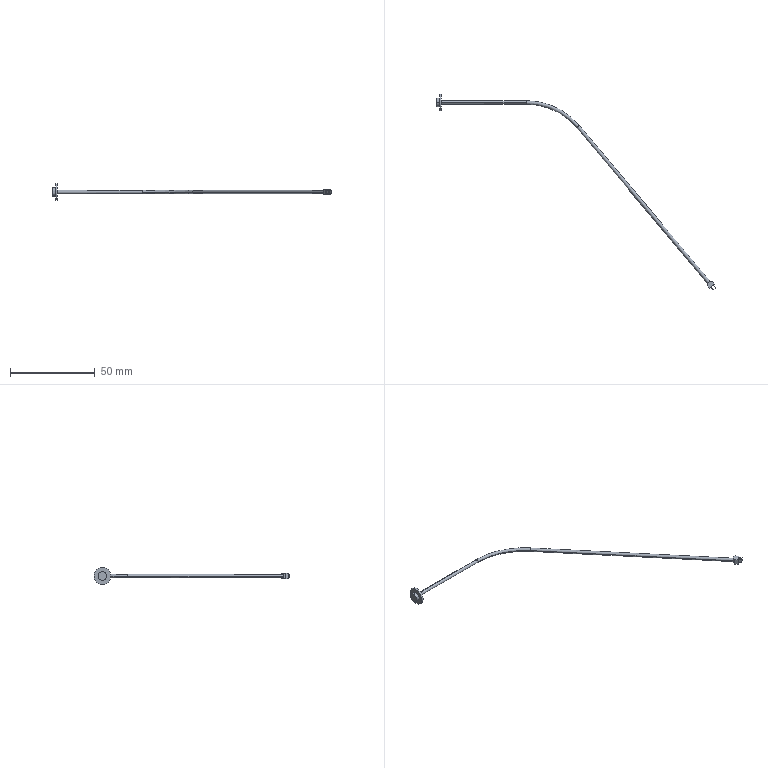Part | SolidWorks | features ICE 2, Revolution 1, Sweep 1 | 1 solid | 32 faces | box 164.795 x 115.719 x 10 mm | volume 796.943 mm3 | plane 22 | cylinder 8 | torus 2 | commonest cylinder face diameters 2 x4 5 x2 10 x2
STEP:
#1=CARTESIAN_POINT('',(53.,1.,0.));
#2=VERTEX_POINT('',#1);
#3=CARTESIAN_POINT('',(53.,0.,-1.));
#4=VERTEX_POINT('',#3);
#5=CARTESIAN_POINT('',(53.,0.,0.));
#6=DIRECTION('',(-1.,0.,0.));
#7=DIRECTION('',(0.,-1.,0.));
#8=AXIS2_PLACEMENT_3D('',#5,#6,#7);
#9=CIRCLE('',#8,1.);
#10=EDGE_CURVE('',#2,#4,#9,.T.);
#11=ORIENTED_EDGE('',*,*,#10,.F.);
#12=CARTESIAN_POINT('',(84.408,-13.646,0.));
#13=VERTEX_POINT('',#12);
#14=CARTESIAN_POINT('',(53.,-40.,0.));
#15=DIRECTION('',(0.,0.,-1.));
#16=DIRECTION('',(-1.,0.,0.));
#17=AXIS2_PLACEMENT_3D('',#14,#15,#16);
#18=CIRCLE('',#17,41.);
#19=EDGE_CURVE('',#2,#13,#18,.T.);
#20=ORIENTED_EDGE('',*,*,#19,.T.);
#21=CARTESIAN_POINT('',(82.876,-14.931,0.));
#22=VERTEX_POINT('',#21);
#23=CARTESIAN_POINT('',(83.642,-14.288,0.));
#24=DIRECTION('',(-0.6428,0.766,0.));
#25=DIRECTION('',(-0.766,-0.6428,0.));
#26=AXIS2_PLACEMENT_3D('',#23,#24,#25);
#27=CIRCLE('',#26,1.);
#28=EDGE_CURVE('',#13,#22,#27,.T.);
#29=ORIENTED_EDGE('',*,*,#28,.T.);
#30=CARTESIAN_POINT('',(53.,-1.,0.));
#31=VERTEX_POINT('',#30);
#32=CARTESIAN_POINT('',(53.,-40.,0.));
#33=DIRECTION('',(0.,0.,-1.));
#34=DIRECTION('',(-1.,0.,0.));
#35=AXIS2_PLACEMENT_3D('',#32,#33,#34);
#36=CIRCLE('',#35,39.);
#37=EDGE_CURVE('',#31,#22,#36,.T.);
#38=ORIENTED_EDGE('',*,*,#37,.F.);
#39=CARTESIAN_POINT('',(53.,0.,0.));
#40=DIRECTION('',(-1.,0.,0.));
#41=DIRECTION('',(0.,-1.,0.));
#42=AXIS2_PLACEMENT_3D('',#39,#40,#41);
#43=CIRCLE('',#42,1.);
#44=EDGE_CURVE('',#4,#31,#43,.T.);
#45=ORIENTED_EDGE('',*,*,#44,.F.);
#46=EDGE_LOOP('',(#11,#20,#29,#38,#45));
#47=FACE_OUTER_BOUND('',#46,.T.);
#48=CARTESIAN_POINT('',(53.,-40.,0.));
#49=DIRECTION('',(0.,0.,-1.));
#50=DIRECTION('',(-1.,0.,0.));
#51=AXIS2_PLACEMENT_3D('',#48,#49,#50);
#52=TOROIDAL_SURFACE('',#51,40.,1.);
#53=ADVANCED_FACE('',(#47),#52,.T.);
#54=CARTESIAN_POINT('',(83.642,-14.288,0.));
#55=DIRECTION('',(-0.6428,0.766,0.));
#56=DIRECTION('',(-0.766,-0.6428,0.));
#57=AXIS2_PLACEMENT_3D('',#54,#55,#56);
#58=CIRCLE('',#57,1.);
#59=EDGE_CURVE('',#22,#13,#58,.T.);
#60=ORIENTED_EDGE('',*,*,#59,.F.);
#61=CARTESIAN_POINT('',(160.01,-106.857,0.));
#62=VERTEX_POINT('',#61);
#63=CARTESIAN_POINT('',(82.876,-14.931,0.));
#64=DIRECTION('',(0.6428,-0.766,0.));
#65=VECTOR('',#64,1000.);
#66=LINE('',#63,#65);
#67=EDGE_CURVE('',#22,#62,#66,.T.);
#68=ORIENTED_EDGE('',*,*,#67,.T.);
#69=CARTESIAN_POINT('',(161.542,-105.571,0.));
#70=VERTEX_POINT('',#69);
#71=CARTESIAN_POINT('',(160.776,-106.214,0.));
#72=DIRECTION('',(-0.6428,0.766,0.));
#73=DIRECTION('',(-0.766,-0.6428,0.));
#74=AXIS2_PLACEMENT_3D('',#71,#72,#73);
#75=CIRCLE('',#74,1.);
#76=EDGE_CURVE('',#62,#70,#75,.T.);
#77=ORIENTED_EDGE('',*,*,#76,.T.);
#78=CARTESIAN_POINT('',(84.408,-13.646,0.));
#79=DIRECTION('',(0.6428,-0.766,0.));
#80=VECTOR('',#79,1000.);
#81=LINE('',#78,#80);
#82=EDGE_CURVE('',#13,#70,#81,.T.);
#83=ORIENTED_EDGE('',*,*,#82,.F.);
#84=EDGE_LOOP('',(#60,#68,#77,#83));
#85=FACE_OUTER_BOUND('',#84,.T.);
#86=CARTESIAN_POINT('',(83.642,-14.288,0.));
#87=DIRECTION('',(0.6428,-0.766,0.));
#88=DIRECTION('',(0.766,0.6428,0.));
#89=AXIS2_PLACEMENT_3D('',#86,#87,#88);
#90=CYLINDRICAL_SURFACE('',#89,1.);
#91=ADVANCED_FACE('',(#85),#90,.T.);
#92=CARTESIAN_POINT('',(3.,0.,1.));
#93=VERTEX_POINT('',#92);
#94=CARTESIAN_POINT('',(3.,0.,-1.));
#95=VERTEX_POINT('',#94);
#96=CARTESIAN_POINT('',(3.,0.,0.));
#97=DIRECTION('',(-1.,0.,0.));
#98=DIRECTION('',(0.,-1.,0.));
#99=AXIS2_PLACEMENT_3D('',#96,#97,#98);
#100=CIRCLE('',#99,1.);
#101=EDGE_CURVE('',#93,#95,#100,.T.);
#102=ORIENTED_EDGE('',*,*,#101,.F.);
#103=CARTESIAN_POINT('',(53.,0.,1.));
#104=VERTEX_POINT('',#103);
#105=CARTESIAN_POINT('',(3.,0.,1.));
#106=DIRECTION('',(1.,0.,0.));
#107=VECTOR('',#106,1000.);
#108=LINE('',#105,#107);
#109=EDGE_CURVE('',#93,#104,#108,.T.);
#110=ORIENTED_EDGE('',*,*,#109,.T.);
#111=CARTESIAN_POINT('',(53.,0.,0.));
#112=DIRECTION('',(-1.,0.,0.));
#113=DIRECTION('',(0.,-1.,0.));
#114=AXIS2_PLACEMENT_3D('',#111,#112,#113);
#115=CIRCLE('',#114,1.);
#116=EDGE_CURVE('',#104,#2,#115,.T.);
#117=ORIENTED_EDGE('',*,*,#116,.T.);
#118=ORIENTED_EDGE('',*,*,#10,.T.);
#119=CARTESIAN_POINT('',(3.,0.,-1.));
#120=DIRECTION('',(1.,0.,0.));
#121=VECTOR('',#120,1000.);
#122=LINE('',#119,#121);
#123=EDGE_CURVE('',#95,#4,#122,.T.);
#124=ORIENTED_EDGE('',*,*,#123,.F.);
#125=EDGE_LOOP('',(#102,#110,#117,#118,#124));
#126=FACE_OUTER_BOUND('',#125,.T.);
#127=CARTESIAN_POINT('',(3.,0.,0.));
#128=DIRECTION('',(1.,0.,0.));
#129=DIRECTION('',(0.,0.,-1.));
#130=AXIS2_PLACEMENT_3D('',#127,#128,#129);
#131=CYLINDRICAL_SURFACE('',#130,1.);
#132=ADVANCED_FACE('',(#126),#131,.T.);
#133=CARTESIAN_POINT('',(3.,0.,5.));
#134=VERTEX_POINT('',#133);
#135=CARTESIAN_POINT('',(3.,0.,-5.));
#136=VERTEX_POINT('',#135);
#137=CARTESIAN_POINT('',(3.,0.,0.));
#138=DIRECTION('',(-1.,0.,0.));
#139=DIRECTION('',(0.,0.,1.));
#140=AXIS2_PLACEMENT_3D('',#137,#138,#139);
#141=CIRCLE('',#140,5.);
#142=EDGE_CURVE('',#134,#136,#141,.T.);
#143=ORIENTED_EDGE('',*,*,#142,.T.);
#144=CARTESIAN_POINT('',(2.,0.,-5.));
#145=VERTEX_POINT('',#144);
#146=CARTESIAN_POINT('',(0.,0.,-5.));
#147=DIRECTION('',(-1.,0.,0.));
#148=VECTOR('',#147,1000.);
#149=LINE('',#146,#148);
#150=EDGE_CURVE('',#136,#145,#149,.T.);
#151=ORIENTED_EDGE('',*,*,#150,.T.);
#152=CARTESIAN_POINT('',(2.,0.,5.));
#153=VERTEX_POINT('',#152);
#154=CARTESIAN_POINT('',(2.,0.,0.));
#155=DIRECTION('',(-1.,0.,0.));
#156=DIRECTION('',(0.,0.,1.));
#157=AXIS2_PLACEMENT_3D('',#154,#155,#156);
#158=CIRCLE('',#157,5.);
#159=EDGE_CURVE('',#153,#145,#158,.T.);
#160=ORIENTED_EDGE('',*,*,#159,.F.);
#161=CARTESIAN_POINT('',(0.,0.,5.));
#162=DIRECTION('',(-1.,0.,0.));
#163=VECTOR('',#162,1000.);
#164=LINE('',#161,#163);
#165=EDGE_CURVE('',#134,#153,#164,.T.);
#166=ORIENTED_EDGE('',*,*,#165,.F.);
#167=EDGE_LOOP('',(#143,#151,#160,#166));
#168=FACE_OUTER_BOUND('',#167,.T.);
#169=CARTESIAN_POINT('',(0.,0.,0.));
#170=DIRECTION('',(-1.,0.,0.));
#171=DIRECTION('',(0.,0.,1.));
#172=AXIS2_PLACEMENT_3D('',#169,#170,#171);
#173=CYLINDRICAL_SURFACE('',#172,5.);
#174=ADVANCED_FACE('',(#168),#173,.T.);
#175=CARTESIAN_POINT('',(2.,0.,2.5));
#176=VERTEX_POINT('',#175);
#177=CARTESIAN_POINT('',(2.,0.,-2.5));
#178=VERTEX_POINT('',#177);
#179=CARTESIAN_POINT('',(2.,0.,0.));
#180=DIRECTION('',(-1.,0.,0.));
#181=DIRECTION('',(0.,0.,1.));
#182=AXIS2_PLACEMENT_3D('',#179,#180,#181);
#183=CIRCLE('',#182,2.5);
#184=EDGE_CURVE('',#176,#178,#183,.T.);
#185=ORIENTED_EDGE('',*,*,#184,.T.);
#186=CARTESIAN_POINT('',(0.,0.,-2.5));
#187=VERTEX_POINT('',#186);
#188=CARTESIAN_POINT('',(0.,0.,-2.5));
#189=DIRECTION('',(-1.,0.,0.));
#190=VECTOR('',#189,1000.);
#191=LINE('',#188,#190);
#192=EDGE_CURVE('',#178,#187,#191,.T.);
#193=ORIENTED_EDGE('',*,*,#192,.T.);
#194=CARTESIAN_POINT('',(0.,0.,2.5));
#195=VERTEX_POINT('',#194);
#196=CARTESIAN_POINT('',(0.,0.,0.));
#197=DIRECTION('',(-1.,0.,0.));
#198=DIRECTION('',(0.,0.,1.));
#199=AXIS2_PLACEMENT_3D('',#196,#197,#198);
#200=CIRCLE('',#199,2.5);
#201=EDGE_CURVE('',#195,#187,#200,.T.);
#202=ORIENTED_EDGE('',*,*,#201,.F.);
#203=CARTESIAN_POINT('',(0.,0.,2.5));
#204=DIRECTION('',(-1.,0.,0.));
#205=VECTOR('',#204,1000.);
#206=LINE('',#203,#205);
#207=EDGE_CURVE('',#176,#195,#206,.T.);
#208=ORIENTED_EDGE('',*,*,#207,.F.);
#209=EDGE_LOOP('',(#185,#193,#202,#208));
#210=FACE_OUTER_BOUND('',#209,.T.);
#211=CARTESIAN_POINT('',(0.,0.,0.));
#212=DIRECTION('',(-1.,0.,0.));
#213=DIRECTION('',(0.,0.,1.));
#214=AXIS2_PLACEMENT_3D('',#211,#212,#213);
#215=CYLINDRICAL_SURFACE('',#214,2.5);
#216=ADVANCED_FACE('',(#210),#215,.T.);
#217=CARTESIAN_POINT('',(161.9,-109.187,1.));
#218=VERTEX_POINT('',#217);
#219=CARTESIAN_POINT('',(161.9,-109.187,-1.));
#220=VERTEX_POINT('',#219);
#221=CARTESIAN_POINT('',(161.9,-109.187,1.));
#222=DIRECTION('',(0.,0.,-1.));
#223=VECTOR('',#222,1000.);
#224=LINE('',#221,#223);
#225=EDGE_CURVE('',#218,#220,#224,.T.);
#226=ORIENTED_EDGE('',*,*,#225,.F.);
#227=CARTESIAN_POINT('',(162.13,-108.994,1.));
#228=VERTEX_POINT('',#227);
#229=CARTESIAN_POINT('',(162.13,-108.994,1.));
#230=DIRECTION('',(-0.766,-0.6428,0.));
#231=VECTOR('',#230,1000.);
#232=LINE('',#229,#231);
#233=EDGE_CURVE('',#228,#218,#232,.T.);
#234=ORIENTED_EDGE('',*,*,#233,.F.);
#235=CARTESIAN_POINT('',(162.13,-108.994,-1.));
#236=VERTEX_POINT('',#235);
#237=CARTESIAN_POINT('',(162.13,-108.994,1.));
#238=DIRECTION('',(0.,0.,-1.));
#239=VECTOR('',#238,1000.);
#240=LINE('',#237,#239);
#241=EDGE_CURVE('',#228,#236,#240,.T.);
#242=ORIENTED_EDGE('',*,*,#241,.T.);
#243=CARTESIAN_POINT('',(162.13,-108.994,-1.));
#244=DIRECTION('',(-0.766,-0.6428,0.));
#245=VECTOR('',#244,1000.);
#246=LINE('',#243,#245);
#247=EDGE_CURVE('',#236,#220,#246,.T.);
#248=ORIENTED_EDGE('',*,*,#247,.T.);
#249=EDGE_LOOP('',(#226,#234,#242,#248));
#250=FACE_BOUND('',#249,.T.);
#251=CARTESIAN_POINT('',(161.173,-109.798,-1.5));
#252=VERTEX_POINT('',#251);
#253=CARTESIAN_POINT('',(164.237,-107.226,-1.5));
#254=VERTEX_POINT('',#253);
#255=CARTESIAN_POINT('',(164.237,-107.226,-1.5));
#256=DIRECTION('',(0.766,0.6428,0.));
#257=VECTOR('',#256,1000.);
#258=LINE('',#255,#257);
#259=EDGE_CURVE('',#252,#254,#258,.T.);
#260=ORIENTED_EDGE('',*,*,#259,.T.);
#261=CARTESIAN_POINT('',(164.237,-107.226,1.5));
#262=VERTEX_POINT('',#261);
#263=CARTESIAN_POINT('',(164.237,-107.226,1.5));
#264=DIRECTION('',(0.,0.,-1.));
#265=VECTOR('',#264,1000.);
#266=LINE('',#263,#265);
#267=EDGE_CURVE('',#262,#254,#266,.T.);
#268=ORIENTED_EDGE('',*,*,#267,.F.);
#269=CARTESIAN_POINT('',(161.173,-109.798,1.5));
#270=VERTEX_POINT('',#269);
#271=CARTESIAN_POINT('',(164.237,-107.226,1.5));
#272=DIRECTION('',(0.766,0.6428,0.));
#273=VECTOR('',#272,1000.);
#274=LINE('',#271,#273);
#275=EDGE_CURVE('',#270,#262,#274,.T.);
#276=ORIENTED_EDGE('',*,*,#275,.F.);
#277=CARTESIAN_POINT('',(161.173,-109.798,1.5));
#278=DIRECTION('',(0.,0.,-1.));
#279=VECTOR('',#278,1000.);
#280=LINE('',#277,#279);
#281=EDGE_CURVE('',#270,#252,#280,.T.);
#282=ORIENTED_EDGE('',*,*,#281,.T.);
#283=EDGE_LOOP('',(#260,#268,#276,#282));
#284=FACE_OUTER_BOUND('',#283,.T.);
#285=CARTESIAN_POINT('',(163.509,-107.837,1.));
#286=VERTEX_POINT('',#285);
#287=CARTESIAN_POINT('',(163.279,-108.03,1.));
#288=VERTEX_POINT('',#287);
#289=CARTESIAN_POINT('',(163.279,-108.03,1.));
#290=DIRECTION('',(-0.766,-0.6428,0.));
#291=VECTOR('',#290,1000.);
#292=LINE('',#289,#291);
#293=EDGE_CURVE('',#286,#288,#292,.T.);
#294=ORIENTED_EDGE('',*,*,#293,.F.);
#295=CARTESIAN_POINT('',(163.509,-107.837,-1.));
#296=VERTEX_POINT('',#295);
#297=CARTESIAN_POINT('',(163.509,-107.837,1.));
#298=DIRECTION('',(0.,0.,-1.));
#299=VECTOR('',#298,1000.);
#300=LINE('',#297,#299);
#301=EDGE_CURVE('',#286,#296,#300,.T.);
#302=ORIENTED_EDGE('',*,*,#301,.T.);
#303=CARTESIAN_POINT('',(163.279,-108.03,-1.));
#304=VERTEX_POINT('',#303);
#305=CARTESIAN_POINT('',(163.279,-108.03,-1.));
#306=DIRECTION('',(-0.766,-0.6428,0.));
#307=VECTOR('',#306,1000.);
#308=LINE('',#305,#307);
#309=EDGE_CURVE('',#296,#304,#308,.T.);
#310=ORIENTED_EDGE('',*,*,#309,.T.);
#311=CARTESIAN_POINT('',(163.279,-108.03,1.));
#312=DIRECTION('',(0.,0.,-1.));
#313=VECTOR('',#312,1000.);
#314=LINE('',#311,#313);
#315=EDGE_CURVE('',#288,#304,#314,.T.);
#316=ORIENTED_EDGE('',*,*,#315,.F.);
#317=EDGE_LOOP('',(#294,#302,#310,#316));
#318=FACE_BOUND('',#317,.T.);
#319=CARTESIAN_POINT('',(164.237,-107.226,1.5));
#320=DIRECTION('',(-0.6428,0.766,0.));
#321=DIRECTION('',(-0.766,-0.6428,0.));
#322=AXIS2_PLACEMENT_3D('',#319,#320,#321);
#323=PLANE('',#322);
#324=ADVANCED_FACE('',(#250,#284,#318),#323,.F.);
#325=ORIENTED_EDGE('',*,*,#201,.T.);
#326=CARTESIAN_POINT('',(0.,0.,0.));
#327=DIRECTION('',(-1.,0.,0.));
#328=DIRECTION('',(0.,0.,1.));
#329=AXIS2_PLACEMENT_3D('',#326,#327,#328);
#330=CIRCLE('',#329,2.5);
#331=EDGE_CURVE('',#187,#195,#330,.T.);
#332=ORIENTED_EDGE('',*,*,#331,.T.);
#333=EDGE_LOOP('',(#325,#332));
#334=FACE_OUTER_BOUND('',#333,.T.);
#335=CARTESIAN_POINT('',(0.,0.,0.));
#336=DIRECTION('',(1.,0.,0.));
#337=DIRECTION('',(0.,0.,-1.));
#338=AXIS2_PLACEMENT_3D('',#335,#336,#337);
#339=PLANE('',#338);
#340=ADVANCED_FACE('',(#334),#339,.F.);
#341=ORIENTED_EDGE('',*,*,#192,.F.);
#342=CARTESIAN_POINT('',(2.,0.,0.));
#343=DIRECTION('',(-1.,0.,0.));
#344=DIRECTION('',(0.,0.,1.));
#345=AXIS2_PLACEMENT_3D('',#342,#343,#344);
#346=CIRCLE('',#345,2.5);
#347=EDGE_CURVE('',#178,#176,#346,.T.);
#348=ORIENTED_EDGE('',*,*,#347,.T.);
#349=ORIENTED_EDGE('',*,*,#207,.T.);
#350=ORIENTED_EDGE('',*,*,#331,.F.);
#351=EDGE_LOOP('',(#341,#348,#349,#350));
#352=FACE_OUTER_BOUND('',#351,.T.);
#353=CARTESIAN_POINT('',(0.,0.,0.));
#354=DIRECTION('',(-1.,0.,0.));
#355=DIRECTION('',(0.,0.,1.));
#356=AXIS2_PLACEMENT_3D('',#353,#354,#355);
#357=CYLINDRICAL_SURFACE('',#356,2.5);
#358=ADVANCED_FACE('',(#352),#357,.T.);
#359=ORIENTED_EDGE('',*,*,#184,.F.);
#360=ORIENTED_EDGE('',*,*,#347,.F.);
#361=EDGE_LOOP('',(#359,#360));
#362=FACE_BOUND('',#361,.T.);
#363=ORIENTED_EDGE('',*,*,#159,.T.);
#364=CARTESIAN_POINT('',(2.,0.,0.));
#365=DIRECTION('',(-1.,0.,0.));
#366=DIRECTION('',(0.,0.,1.));
#367=AXIS2_PLACEMENT_3D('',#364,#365,#366);
#368=CIRCLE('',#367,5.);
#369=EDGE_CURVE('',#145,#153,#368,.T.);
#370=ORIENTED_EDGE('',*,*,#369,.T.);
#371=EDGE_LOOP('',(#363,#370));
#372=FACE_OUTER_BOUND('',#371,.T.);
#373=CARTESIAN_POINT('',(2.,2.5,0.));
#374=DIRECTION('',(1.,0.,0.));
#375=DIRECTION('',(0.,0.,-1.));
#376=AXIS2_PLACEMENT_3D('',#373,#374,#375);
#377=PLANE('',#376);
#378=ADVANCED_FACE('',(#362,#372),#377,.F.);
#379=ORIENTED_EDGE('',*,*,#150,.F.);
#380=CARTESIAN_POINT('',(3.,0.,0.));
#381=DIRECTION('',(-1.,0.,0.));
#382=DIRECTION('',(0.,0.,1.));
#383=AXIS2_PLACEMENT_3D('',#380,#381,#382);
#384=CIRCLE('',#383,5.);
#385=EDGE_CURVE('',#136,#134,#384,.T.);
#386=ORIENTED_EDGE('',*,*,#385,.T.);
#387=ORIENTED_EDGE('',*,*,#165,.T.);
#388=ORIENTED_EDGE('',*,*,#369,.F.);
#389=EDGE_LOOP('',(#379,#386,#387,#388));
#390=FACE_OUTER_BOUND('',#389,.T.);
#391=CARTESIAN_POINT('',(0.,0.,0.));
#392=DIRECTION('',(-1.,0.,0.));
#393=DIRECTION('',(0.,0.,1.));
#394=AXIS2_PLACEMENT_3D('',#391,#392,#393);
#395=CYLINDRICAL_SURFACE('',#394,5.);
#396=ADVANCED_FACE('',(#390),#395,.T.);
#397=CARTESIAN_POINT('',(3.,0.,0.));
#398=DIRECTION('',(-1.,0.,0.));
#399=DIRECTION('',(0.,-1.,0.));
#400=AXIS2_PLACEMENT_3D('',#397,#398,#399);
#401=CIRCLE('',#400,1.);
#402=EDGE_CURVE('',#95,#93,#401,.T.);
#403=ORIENTED_EDGE('',*,*,#402,.T.);
#404=ORIENTED_EDGE('',*,*,#101,.T.);
#405=EDGE_LOOP('',(#403,#404));
#406=FACE_BOUND('',#405,.T.);
#407=ORIENTED_EDGE('',*,*,#142,.F.);
#408=ORIENTED_EDGE('',*,*,#385,.F.);
#409=EDGE_LOOP('',(#407,#408));
#410=FACE_OUTER_BOUND('',#409,.T.);
#411=CARTESIAN_POINT('',(3.,5.,0.));
#412=DIRECTION('',(-1.,0.,0.));
#413=DIRECTION('',(0.,0.,1.));
#414=AXIS2_PLACEMENT_3D('',#411,#412,#413);
#415=PLANE('',#414);
#416=ADVANCED_FACE('',(#406,#410),#415,.F.);
#417=ORIENTED_EDGE('',*,*,#67,.F.);
#418=ORIENTED_EDGE('',*,*,#28,.F.);
#419=ORIENTED_EDGE('',*,*,#82,.T.);
#420=CARTESIAN_POINT('',(160.776,-106.214,0.));
#421=DIRECTION('',(-0.6428,0.766,0.));
#422=DIRECTION('',(-0.766,-0.6428,0.));
#423=AXIS2_PLACEMENT_3D('',#420,#421,#422);
#424=CIRCLE('',#423,1.);
#425=EDGE_CURVE('',#70,#62,#424,.T.);
#426=ORIENTED_EDGE('',*,*,#425,.T.);
#427=EDGE_LOOP('',(#417,#418,#419,#426));
#428=FACE_OUTER_BOUND('',#427,.T.);
#429=CARTESIAN_POINT('',(83.642,-14.288,0.));
#430=DIRECTION('',(0.6428,-0.766,0.));
#431=DIRECTION('',(0.766,0.6428,0.));
#432=AXIS2_PLACEMENT_3D('',#429,#430,#431);
#433=CYLINDRICAL_SURFACE('',#432,1.);
#434=ADVANCED_FACE('',(#428),#433,.T.);
#435=ORIENTED_EDGE('',*,*,#19,.F.);
#436=ORIENTED_EDGE('',*,*,#116,.F.);
#437=CARTESIAN_POINT('',(53.,0.,0.));
#438=DIRECTION('',(-1.,0.,0.));
#439=DIRECTION('',(0.,-1.,0.));
#440=AXIS2_PLACEMENT_3D('',#437,#438,#439);
#441=CIRCLE('',#440,1.);
#442=EDGE_CURVE('',#31,#104,#441,.T.);
#443=ORIENTED_EDGE('',*,*,#442,.F.);
#444=ORIENTED_EDGE('',*,*,#37,.T.);
#445=ORIENTED_EDGE('',*,*,#59,.T.);
#446=EDGE_LOOP('',(#435,#436,#443,#444,#445));
#447=FACE_OUTER_BOUND('',#446,.T.);
#448=CARTESIAN_POINT('',(53.,-40.,0.));
#449=DIRECTION('',(0.,0.,-1.));
#450=DIRECTION('',(-1.,0.,0.));
#451=AXIS2_PLACEMENT_3D('',#448,#449,#450);
#452=TOROIDAL_SURFACE('',#451,40.,1.);
#453=ADVANCED_FACE('',(#447),#452,.T.);
#454=ORIENTED_EDGE('',*,*,#109,.F.);
#455=ORIENTED_EDGE('',*,*,#402,.F.);
#456=ORIENTED_EDGE('',*,*,#123,.T.);
#457=ORIENTED_EDGE('',*,*,#44,.T.);
#458=ORIENTED_EDGE('',*,*,#442,.T.);
#459=EDGE_LOOP('',(#454,#455,#456,#457,#458));
#460=FACE_OUTER_BOUND('',#459,.T.);
#461=CARTESIAN_POINT('',(3.,0.,0.));
#462=DIRECTION('',(1.,0.,0.));
#463=DIRECTION('',(0.,0.,-1.));
#464=AXIS2_PLACEMENT_3D('',#461,#462,#463);
#465=CYLINDRICAL_SURFACE('',#464,1.);
#466=ADVANCED_FACE('',(#460),#465,.T.);
#467=ORIENTED_EDGE('',*,*,#76,.F.);
#468=CARTESIAN_POINT('',(160.01,-106.857,1.5));
#469=VERTEX_POINT('',#468);
#470=CARTESIAN_POINT('',(160.01,-106.857,1.5));
#471=DIRECTION('',(0.,0.,-1.));
#472=VECTOR('',#471,1000.);
#473=LINE('',#470,#472);
#474=EDGE_CURVE('',#469,#62,#473,.T.);
#475=ORIENTED_EDGE('',*,*,#474,.F.);
#476=CARTESIAN_POINT('',(161.542,-105.571,1.5));
#477=VERTEX_POINT('',#476);
#478=CARTESIAN_POINT('',(160.01,-106.857,1.5));
#479=DIRECTION('',(-0.766,-0.6428,0.));
#480=VECTOR('',#479,1000.);
#481=LINE('',#478,#480);
#482=EDGE_CURVE('',#477,#469,#481,.T.);
#483=ORIENTED_EDGE('',*,*,#482,.F.);
#484=CARTESIAN_POINT('',(161.542,-105.571,1.5));
#485=DIRECTION('',(0.,0.,-1.));
#486=VECTOR('',#485,1000.);
#487=LINE('',#484,#486);
#488=EDGE_CURVE('',#477,#70,#487,.T.);
#489=ORIENTED_EDGE('',*,*,#488,.T.);
#490=EDGE_LOOP('',(#467,#475,#483,#489));
#491=FACE_OUTER_BOUND('',#490,.T.);
#492=CARTESIAN_POINT('',(160.01,-106.857,1.5));
#493=DIRECTION('',(0.6428,-0.766,0.));
#494=DIRECTION('',(0.766,0.6428,0.));
#495=AXIS2_PLACEMENT_3D('',#492,#493,#494);
#496=PLANE('',#495);
#497=ADVANCED_FACE('',(#491),#496,.F.);
#498=CARTESIAN_POINT('',(162.951,-105.694,-1.5));
#499=VERTEX_POINT('',#498);
#500=CARTESIAN_POINT('',(161.542,-105.571,-1.5));
#501=VERTEX_POINT('',#500);
#502=CARTESIAN_POINT('',(161.542,-105.571,-1.5));
#503=DIRECTION('',(-0.9962,0.08716,0.));
#504=VECTOR('',#503,1000.);
#505=LINE('',#502,#504);
#506=EDGE_CURVE('',#499,#501,#505,.T.);
#507=ORIENTED_EDGE('',*,*,#506,.T.);
#508=CARTESIAN_POINT('',(161.542,-105.571,1.5));
#509=DIRECTION('',(0.,0.,-1.));
#510=VECTOR('',#509,1000.);
#511=LINE('',#508,#510);
#512=EDGE_CURVE('',#70,#501,#511,.T.);
#513=ORIENTED_EDGE('',*,*,#512,.F.);
#514=ORIENTED_EDGE('',*,*,#488,.F.);
#515=CARTESIAN_POINT('',(162.951,-105.694,1.5));
#516=VERTEX_POINT('',#515);
#517=CARTESIAN_POINT('',(161.542,-105.571,1.5));
#518=DIRECTION('',(-0.9962,0.08716,0.));
#519=VECTOR('',#518,1000.);
#520=LINE('',#517,#519);
#521=EDGE_CURVE('',#516,#477,#520,.T.);
#522=ORIENTED_EDGE('',*,*,#521,.F.);
#523=CARTESIAN_POINT('',(162.951,-105.694,1.5));
#524=DIRECTION('',(0.,0.,-1.));
#525=VECTOR('',#524,1000.);
#526=LINE('',#523,#525);
#527=EDGE_CURVE('',#516,#499,#526,.T.);
#528=ORIENTED_EDGE('',*,*,#527,.T.);
#529=EDGE_LOOP('',(#507,#513,#514,#522,#528));
#530=FACE_OUTER_BOUND('',#529,.T.);
#531=CARTESIAN_POINT('',(161.542,-105.571,1.5));
#532=DIRECTION('',(-0.08716,-0.9962,0.));
#533=DIRECTION('',(0.9962,-0.08716,0.));
#534=AXIS2_PLACEMENT_3D('',#531,#532,#533);
#535=PLANE('',#534);
#536=ADVANCED_FACE('',(#530),#535,.F.);
#537=ORIENTED_EDGE('',*,*,#425,.F.);
#538=ORIENTED_EDGE('',*,*,#512,.T.);
#539=CARTESIAN_POINT('',(160.01,-106.857,-1.5));
#540=VERTEX_POINT('',#539);
#541=CARTESIAN_POINT('',(160.01,-106.857,-1.5));
#542=DIRECTION('',(-0.766,-0.6428,0.));
#543=VECTOR('',#542,1000.);
#544=LINE('',#541,#543);
#545=EDGE_CURVE('',#501,#540,#544,.T.);
#546=ORIENTED_EDGE('',*,*,#545,.T.);
#547=CARTESIAN_POINT('',(160.01,-106.857,1.5));
#548=DIRECTION('',(0.,0.,-1.));
#549=VECTOR('',#548,1000.);
#550=LINE('',#547,#549);
#551=EDGE_CURVE('',#62,#540,#550,.T.);
#552=ORIENTED_EDGE('',*,*,#551,.F.);
#553=EDGE_LOOP('',(#537,#538,#546,#552));
#554=FACE_OUTER_BOUND('',#553,.T.);
#555=CARTESIAN_POINT('',(160.01,-106.857,1.5));
#556=DIRECTION('',(0.6428,-0.766,0.));
#557=DIRECTION('',(0.766,0.6428,0.));
#558=AXIS2_PLACEMENT_3D('',#555,#556,#557);
#559=PLANE('',#558);
#560=ADVANCED_FACE('',(#554),#559,.F.);
#561=CARTESIAN_POINT('',(159.887,-108.265,-1.5));
#562=VERTEX_POINT('',#561);
#563=CARTESIAN_POINT('',(160.01,-106.857,-1.5));
#564=DIRECTION('',(-0.08716,-0.9962,0.));
#565=VECTOR('',#564,1000.);
#566=LINE('',#563,#565);
#567=EDGE_CURVE('',#540,#562,#566,.T.);
#568=ORIENTED_EDGE('',*,*,#567,.T.);
#569=CARTESIAN_POINT('',(159.887,-108.265,1.5));
#570=VERTEX_POINT('',#569);
#571=CARTESIAN_POINT('',(159.887,-108.265,1.5));
#572=DIRECTION('',(0.,0.,-1.));
#573=VECTOR('',#572,1000.);
#574=LINE('',#571,#573);
#575=EDGE_CURVE('',#570,#562,#574,.T.);
#576=ORIENTED_EDGE('',*,*,#575,.F.);
#577=CARTESIAN_POINT('',(160.01,-106.857,1.5));
#578=DIRECTION('',(-0.08716,-0.9962,0.));
#579=VECTOR('',#578,1000.);
#580=LINE('',#577,#579);
#581=EDGE_CURVE('',#469,#570,#580,.T.);
#582=ORIENTED_EDGE('',*,*,#581,.F.);
#583=ORIENTED_EDGE('',*,*,#474,.T.);
#584=ORIENTED_EDGE('',*,*,#551,.T.);
#585=EDGE_LOOP('',(#568,#576,#582,#583,#584));
#586=FACE_OUTER_BOUND('',#585,.T.);
#587=CARTESIAN_POINT('',(160.01,-106.857,1.5));
#588=DIRECTION('',(0.9962,-0.08716,0.));
#589=DIRECTION('',(0.08716,0.9962,0.));
#590=AXIS2_PLACEMENT_3D('',#587,#588,#589);
#591=PLANE('',#590);
#592=ADVANCED_FACE('',(#586),#591,.F.);
#593=CARTESIAN_POINT('',(159.887,-108.265,-1.5));
#594=DIRECTION('',(0.6428,-0.766,0.));
#595=VECTOR('',#594,1000.);
#596=LINE('',#593,#595);
#597=EDGE_CURVE('',#562,#252,#596,.T.);
#598=ORIENTED_EDGE('',*,*,#597,.T.);
#599=ORIENTED_EDGE('',*,*,#281,.F.);
#600=CARTESIAN_POINT('',(159.887,-108.265,1.5));
#601=DIRECTION('',(0.6428,-0.766,0.));
#602=VECTOR('',#601,1000.);
#603=LINE('',#600,#602);
#604=EDGE_CURVE('',#570,#270,#603,.T.);
#605=ORIENTED_EDGE('',*,*,#604,.F.);
#606=ORIENTED_EDGE('',*,*,#575,.T.);
#607=EDGE_LOOP('',(#598,#599,#605,#606));
#608=FACE_OUTER_BOUND('',#607,.T.);
#609=CARTESIAN_POINT('',(159.887,-108.265,1.5));
#610=DIRECTION('',(0.766,0.6428,0.));
#611=DIRECTION('',(-0.6428,0.766,0.));
#612=AXIS2_PLACEMENT_3D('',#609,#610,#611);
#613=PLANE('',#612);
#614=ADVANCED_FACE('',(#608),#613,.F.);
#615=CARTESIAN_POINT('',(162.951,-105.694,-1.5));
#616=DIRECTION('',(-0.6428,0.766,0.));
#617=VECTOR('',#616,1000.);
#618=LINE('',#615,#617);
#619=EDGE_CURVE('',#254,#499,#618,.T.);
#620=ORIENTED_EDGE('',*,*,#619,.T.);
#621=ORIENTED_EDGE('',*,*,#527,.F.);
#622=CARTESIAN_POINT('',(162.951,-105.694,1.5));
#623=DIRECTION('',(-0.6428,0.766,0.));
#624=VECTOR('',#623,1000.);
#625=LINE('',#622,#624);
#626=EDGE_CURVE('',#262,#516,#625,.T.);
#627=ORIENTED_EDGE('',*,*,#626,.F.);
#628=ORIENTED_EDGE('',*,*,#267,.T.);
#629=EDGE_LOOP('',(#620,#621,#627,#628));
#630=FACE_OUTER_BOUND('',#629,.T.);
#631=CARTESIAN_POINT('',(162.951,-105.694,1.5));
#632=DIRECTION('',(-0.766,-0.6428,0.));
#633=DIRECTION('',(0.6428,-0.766,0.));
#634=AXIS2_PLACEMENT_3D('',#631,#632,#633);
#635=PLANE('',#634);
#636=ADVANCED_FACE('',(#630),#635,.F.);
#637=ORIENTED_EDGE('',*,*,#521,.T.);
#638=ORIENTED_EDGE('',*,*,#482,.T.);
#639=ORIENTED_EDGE('',*,*,#581,.T.);
#640=ORIENTED_EDGE('',*,*,#604,.T.);
#641=ORIENTED_EDGE('',*,*,#275,.T.);
#642=ORIENTED_EDGE('',*,*,#626,.T.);
#643=EDGE_LOOP('',(#637,#638,#639,#640,#641,#642));
#644=FACE_OUTER_BOUND('',#643,.T.);
#645=CARTESIAN_POINT('',(0.,0.,1.5));
#646=DIRECTION('',(0.,0.,-1.));
#647=DIRECTION('',(-1.,0.,0.));
#648=AXIS2_PLACEMENT_3D('',#645,#646,#647);
#649=PLANE('',#648);
#650=ADVANCED_FACE('',(#644),#649,.F.);
#651=ORIENTED_EDGE('',*,*,#506,.F.);
#652=ORIENTED_EDGE('',*,*,#619,.F.);
#653=ORIENTED_EDGE('',*,*,#259,.F.);
#654=ORIENTED_EDGE('',*,*,#597,.F.);
#655=ORIENTED_EDGE('',*,*,#567,.F.);
#656=ORIENTED_EDGE('',*,*,#545,.F.);
#657=EDGE_LOOP('',(#651,#652,#653,#654,#655,#656));
#658=FACE_OUTER_BOUND('',#657,.T.);
#659=CARTESIAN_POINT('',(0.,0.,-1.5));
#660=DIRECTION('',(0.,0.,-1.));
#661=DIRECTION('',(-1.,0.,0.));
#662=AXIS2_PLACEMENT_3D('',#659,#660,#661);
#663=PLANE('',#662);
#664=ADVANCED_FACE('',(#658),#663,.T.);
#665=CARTESIAN_POINT('',(164.565,-109.562,-1.));
#666=VERTEX_POINT('',#665);
#667=CARTESIAN_POINT('',(164.565,-109.562,-1.));
#668=DIRECTION('',(0.6428,-0.766,0.));
#669=VECTOR('',#668,1000.);
#670=LINE('',#667,#669);
#671=EDGE_CURVE('',#304,#666,#670,.T.);
#672=ORIENTED_EDGE('',*,*,#671,.T.);
#673=CARTESIAN_POINT('',(164.565,-109.562,1.));
#674=VERTEX_POINT('',#673);
#675=CARTESIAN_POINT('',(164.565,-109.562,1.));
#676=DIRECTION('',(0.,0.,-1.));
#677=VECTOR('',#676,1000.);
#678=LINE('',#675,#677);
#679=EDGE_CURVE('',#674,#666,#678,.T.);
#680=ORIENTED_EDGE('',*,*,#679,.F.);
#681=CARTESIAN_POINT('',(164.565,-109.562,1.));
#682=DIRECTION('',(0.6428,-0.766,0.));
#683=VECTOR('',#682,1000.);
#684=LINE('',#681,#683);
#685=EDGE_CURVE('',#288,#674,#684,.T.);
#686=ORIENTED_EDGE('',*,*,#685,.F.);
#687=ORIENTED_EDGE('',*,*,#315,.T.);
#688=EDGE_LOOP('',(#672,#680,#686,#687));
#689=FACE_OUTER_BOUND('',#688,.T.);
#690=CARTESIAN_POINT('',(164.565,-109.562,1.));
#691=DIRECTION('',(0.766,0.6428,0.));
#692=DIRECTION('',(-0.6428,0.766,0.));
#693=AXIS2_PLACEMENT_3D('',#690,#691,#692);
#694=PLANE('',#693);
#695=ADVANCED_FACE('',(#689),#694,.F.);
#696=CARTESIAN_POINT('',(164.795,-109.369,-1.));
#697=VERTEX_POINT('',#696);
#698=CARTESIAN_POINT('',(164.795,-109.369,-1.));
#699=DIRECTION('',(0.766,0.6428,0.));
#700=VECTOR('',#699,1000.);
#701=LINE('',#698,#700);
#702=EDGE_CURVE('',#666,#697,#701,.T.);
#703=ORIENTED_EDGE('',*,*,#702,.T.);
#704=CARTESIAN_POINT('',(164.795,-109.369,1.));
#705=VERTEX_POINT('',#704);
#706=CARTESIAN_POINT('',(164.795,-109.369,1.));
#707=DIRECTION('',(0.,0.,-1.));
#708=VECTOR('',#707,1000.);
#709=LINE('',#706,#708);
#710=EDGE_CURVE('',#705,#697,#709,.T.);
#711=ORIENTED_EDGE('',*,*,#710,.F.);
#712=CARTESIAN_POINT('',(164.795,-109.369,1.));
#713=DIRECTION('',(0.766,0.6428,0.));
#714=VECTOR('',#713,1000.);
#715=LINE('',#712,#714);
#716=EDGE_CURVE('',#674,#705,#715,.T.);
#717=ORIENTED_EDGE('',*,*,#716,.F.);
#718=ORIENTED_EDGE('',*,*,#679,.T.);
#719=EDGE_LOOP('',(#703,#711,#717,#718));
#720=FACE_OUTER_BOUND('',#719,.T.);
#721=CARTESIAN_POINT('',(164.795,-109.369,1.));
#722=DIRECTION('',(-0.6428,0.766,0.));
#723=DIRECTION('',(-0.766,-0.6428,0.));
#724=AXIS2_PLACEMENT_3D('',#721,#722,#723);
#725=PLANE('',#724);
#726=ADVANCED_FACE('',(#720),#725,.F.);
#727=CARTESIAN_POINT('',(163.509,-107.837,-1.));
#728=DIRECTION('',(-0.6428,0.766,0.));
#729=VECTOR('',#728,1000.);
#730=LINE('',#727,#729);
#731=EDGE_CURVE('',#697,#296,#730,.T.);
#732=ORIENTED_EDGE('',*,*,#731,.T.);
#733=ORIENTED_EDGE('',*,*,#301,.F.);
#734=CARTESIAN_POINT('',(163.509,-107.837,1.));
#735=DIRECTION('',(-0.6428,0.766,0.));
#736=VECTOR('',#735,1000.);
#737=LINE('',#734,#736);
#738=EDGE_CURVE('',#705,#286,#737,.T.);
#739=ORIENTED_EDGE('',*,*,#738,.F.);
#740=ORIENTED_EDGE('',*,*,#710,.T.);
#741=EDGE_LOOP('',(#732,#733,#739,#740));
#742=FACE_OUTER_BOUND('',#741,.T.);
#743=CARTESIAN_POINT('',(163.509,-107.837,1.));
#744=DIRECTION('',(-0.766,-0.6428,0.));
#745=DIRECTION('',(0.6428,-0.766,0.));
#746=AXIS2_PLACEMENT_3D('',#743,#744,#745);
#747=PLANE('',#746);
#748=ADVANCED_FACE('',(#742),#747,.F.);
#749=ORIENTED_EDGE('',*,*,#293,.T.);
#750=ORIENTED_EDGE('',*,*,#685,.T.);
#751=ORIENTED_EDGE('',*,*,#716,.T.);
#752=ORIENTED_EDGE('',*,*,#738,.T.);
#753=EDGE_LOOP('',(#749,#750,#751,#752));
#754=FACE_OUTER_BOUND('',#753,.T.);
#755=CARTESIAN_POINT('',(0.,0.,1.));
#756=DIRECTION('',(0.,0.,-1.));
#757=DIRECTION('',(-1.,0.,0.));
#758=AXIS2_PLACEMENT_3D('',#755,#756,#757);
#759=PLANE('',#758);
#760=ADVANCED_FACE('',(#754),#759,.F.);
#761=ORIENTED_EDGE('',*,*,#309,.F.);
#762=ORIENTED_EDGE('',*,*,#731,.F.);
#763=ORIENTED_EDGE('',*,*,#702,.F.);
#764=ORIENTED_EDGE('',*,*,#671,.F.);
#765=EDGE_LOOP('',(#761,#762,#763,#764));
#766=FACE_OUTER_BOUND('',#765,.T.);
#767=CARTESIAN_POINT('',(0.,0.,-1.));
#768=DIRECTION('',(0.,0.,-1.));
#769=DIRECTION('',(-1.,0.,0.));
#770=AXIS2_PLACEMENT_3D('',#767,#768,#769);
#771=PLANE('',#770);
#772=ADVANCED_FACE('',(#766),#771,.T.);
#773=CARTESIAN_POINT('',(163.416,-110.526,-1.));
#774=VERTEX_POINT('',#773);
#775=CARTESIAN_POINT('',(163.416,-110.526,-1.));
#776=DIRECTION('',(-0.6428,0.766,0.));
#777=VECTOR('',#776,1000.);
#778=LINE('',#775,#777);
#779=EDGE_CURVE('',#774,#236,#778,.T.);
#780=ORIENTED_EDGE('',*,*,#779,.T.);
#781=ORIENTED_EDGE('',*,*,#241,.F.);
#782=CARTESIAN_POINT('',(163.416,-110.526,1.));
#783=VERTEX_POINT('',#782);
#784=CARTESIAN_POINT('',(163.416,-110.526,1.));
#785=DIRECTION('',(-0.6428,0.766,0.));
#786=VECTOR('',#785,1000.);
#787=LINE('',#784,#786);
#788=EDGE_CURVE('',#783,#228,#787,.T.);
#789=ORIENTED_EDGE('',*,*,#788,.F.);
#790=CARTESIAN_POINT('',(163.416,-110.526,1.));
#791=DIRECTION('',(0.,0.,-1.));
#792=VECTOR('',#791,1000.);
#793=LINE('',#790,#792);
#794=EDGE_CURVE('',#783,#774,#793,.T.);
#795=ORIENTED_EDGE('',*,*,#794,.T.);
#796=EDGE_LOOP('',(#780,#781,#789,#795));
#797=FACE_OUTER_BOUND('',#796,.T.);
#798=CARTESIAN_POINT('',(163.416,-110.526,1.));
#799=DIRECTION('',(-0.766,-0.6428,0.));
#800=DIRECTION('',(0.6428,-0.766,0.));
#801=AXIS2_PLACEMENT_3D('',#798,#799,#800);
#802=PLANE('',#801);
#803=ADVANCED_FACE('',(#797),#802,.F.);
#804=CARTESIAN_POINT('',(163.186,-110.719,-1.));
#805=VERTEX_POINT('',#804);
#806=CARTESIAN_POINT('',(161.9,-109.187,-1.));
#807=DIRECTION('',(0.6428,-0.766,0.));
#808=VECTOR('',#807,1000.);
#809=LINE('',#806,#808);
#810=EDGE_CURVE('',#220,#805,#809,.T.);
#811=ORIENTED_EDGE('',*,*,#810,.T.);
#812=CARTESIAN_POINT('',(163.186,-110.719,1.));
#813=VERTEX_POINT('',#812);
#814=CARTESIAN_POINT('',(163.186,-110.719,1.));
#815=DIRECTION('',(0.,0.,-1.));
#816=VECTOR('',#815,1000.);
#817=LINE('',#814,#816);
#818=EDGE_CURVE('',#813,#805,#817,.T.);
#819=ORIENTED_EDGE('',*,*,#818,.F.);
#820=CARTESIAN_POINT('',(161.9,-109.187,1.));
#821=DIRECTION('',(0.6428,-0.766,0.));
#822=VECTOR('',#821,1000.);
#823=LINE('',#820,#822);
#824=EDGE_CURVE('',#218,#813,#823,.T.);
#825=ORIENTED_EDGE('',*,*,#824,.F.);
#826=ORIENTED_EDGE('',*,*,#225,.T.);
#827=EDGE_LOOP('',(#811,#819,#825,#826));
#828=FACE_OUTER_BOUND('',#827,.T.);
#829=CARTESIAN_POINT('',(161.9,-109.187,1.));
#830=DIRECTION('',(0.766,0.6428,0.));
#831=DIRECTION('',(-0.6428,0.766,0.));
#832=AXIS2_PLACEMENT_3D('',#829,#830,#831);
#833=PLANE('',#832);
#834=ADVANCED_FACE('',(#828),#833,.F.);
#835=CARTESIAN_POINT('',(163.186,-110.719,-1.));
#836=DIRECTION('',(0.766,0.6428,0.));
#837=VECTOR('',#836,1000.);
#838=LINE('',#835,#837);
#839=EDGE_CURVE('',#805,#774,#838,.T.);
#840=ORIENTED_EDGE('',*,*,#839,.T.);
#841=ORIENTED_EDGE('',*,*,#794,.F.);
#842=CARTESIAN_POINT('',(163.186,-110.719,1.));
#843=DIRECTION('',(0.766,0.6428,0.));
#844=VECTOR('',#843,1000.);
#845=LINE('',#842,#844);
#846=EDGE_CURVE('',#813,#783,#845,.T.);
#847=ORIENTED_EDGE('',*,*,#846,.F.);
#848=ORIENTED_EDGE('',*,*,#818,.T.);
#849=EDGE_LOOP('',(#840,#841,#847,#848));
#850=FACE_OUTER_BOUND('',#849,.T.);
#851=CARTESIAN_POINT('',(163.186,-110.719,1.));
#852=DIRECTION('',(-0.6428,0.766,0.));
#853=DIRECTION('',(-0.766,-0.6428,0.));
#854=AXIS2_PLACEMENT_3D('',#851,#852,#853);
#855=PLANE('',#854);
#856=ADVANCED_FACE('',(#850),#855,.F.);
#857=ORIENTED_EDGE('',*,*,#788,.T.);
#858=ORIENTED_EDGE('',*,*,#233,.T.);
#859=ORIENTED_EDGE('',*,*,#824,.T.);
#860=ORIENTED_EDGE('',*,*,#846,.T.);
#861=EDGE_LOOP('',(#857,#858,#859,#860));
#862=FACE_OUTER_BOUND('',#861,.T.);
#863=CARTESIAN_POINT('',(0.,0.,1.));
#864=DIRECTION('',(0.,0.,1.));
#865=DIRECTION('',(1.,0.,0.));
#866=AXIS2_PLACEMENT_3D('',#863,#864,#865);
#867=PLANE('',#866);
#868=ADVANCED_FACE('',(#862),#867,.T.);
#869=ORIENTED_EDGE('',*,*,#779,.F.);
#870=ORIENTED_EDGE('',*,*,#839,.F.);
#871=ORIENTED_EDGE('',*,*,#810,.F.);
#872=ORIENTED_EDGE('',*,*,#247,.F.);
#873=EDGE_LOOP('',(#869,#870,#871,#872));
#874=FACE_OUTER_BOUND('',#873,.T.);
#875=CARTESIAN_POINT('',(0.,0.,-1.));
#876=DIRECTION('',(0.,0.,1.));
#877=DIRECTION('',(1.,0.,0.));
#878=AXIS2_PLACEMENT_3D('',#875,#876,#877);
#879=PLANE('',#878);
#880=ADVANCED_FACE('',(#874),#879,.F.);
#881=CLOSED_SHELL('',(#53,#91,#132,#174,#216,#324,#340,#358,#378,#396,#416,#434,#453,#466,#497,#536,#560,#592,#614,#636,#650,#664,#695,#726,#748,#760,#772,#803,#834,#856,#868,#880));
#882=MANIFOLD_SOLID_BREP('',#881);
#883=CARTESIAN_POINT('',(0.,0.,0.));
#884=DIRECTION('',(0.,0.,1.));
#885=DIRECTION('',(1.,0.,0.));
#886=AXIS2_PLACEMENT_3D('',#883,#884,#885);
#887=(LENGTH_UNIT()NAMED_UNIT(*)SI_UNIT(.MILLI.,.METRE.));
#888=UNCERTAINTY_MEASURE_WITH_UNIT(LENGTH_MEASURE(0.00001),#887,'','');
#889=(NAMED_UNIT(*)PLANE_ANGLE_UNIT()SI_UNIT($,.RADIAN.));
#890=(NAMED_UNIT(*)SI_UNIT($,.STERADIAN.)SOLID_ANGLE_UNIT());
#891=(GEOMETRIC_REPRESENTATION_CONTEXT(3)GLOBAL_UNCERTAINTY_ASSIGNED_CONTEXT((#888))GLOBAL_UNIT_ASSIGNED_CONTEXT((#887,#889,#890))REPRESENTATION_CONTEXT('',''));
#892=ADVANCED_BREP_SHAPE_REPRESENTATION('',(#882,#886),#891);